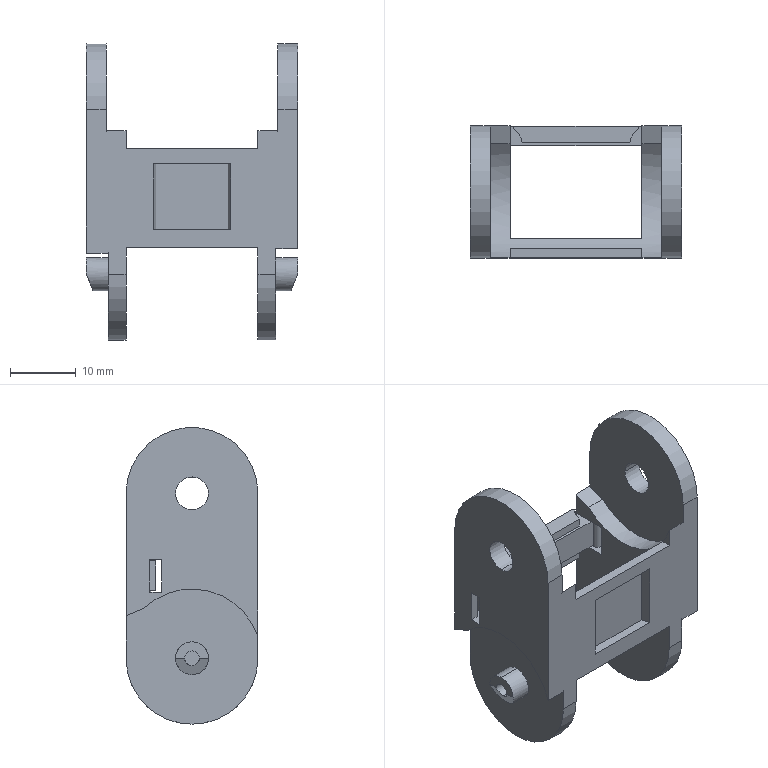Part | STEP file | 1 solid | 95 faces | box 32 x 20 x 45 mm | volume 6516 mm3 | plane 55 | cylinder 40 | commonest cylinder face diameters 5 x8 0.4 x6 1.7 x6 20 x6 2.222 x4 6.708 x4